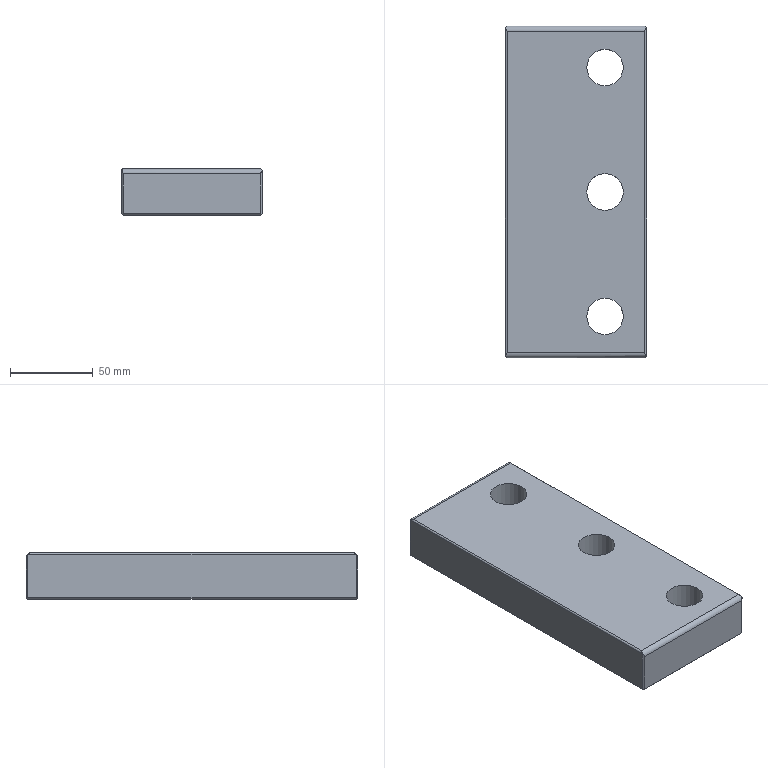Part | NX | features solid 2 | 1 solid | 21 faces | box 85 x 200 x 28 mm | volume 443266 mm3 | plane 15 | cylinder 6 | commonest cylinder face diameters 22 x3 6 x2 2 x1
STEP:
#1=CARTESIAN_POINT('',(590.,131.,-159.));
#2=VERTEX_POINT('',#1);
#3=CARTESIAN_POINT('',(590.,131.,-133.));
#4=VERTEX_POINT('',#3);
#5=CARTESIAN_POINT('',(590.,131.,-132.));
#6=DIRECTION('',(0.,0.,1.));
#7=VECTOR('',#6,1000.);
#8=LINE('',#5,#7);
#9=EDGE_CURVE('',#2,#4,#8,.T.);
#10=ORIENTED_EDGE('',*,*,#9,.T.);
#11=CARTESIAN_POINT('',(590.,329.,-133.));
#12=VERTEX_POINT('',#11);
#13=CARTESIAN_POINT('',(590.,350.,-133.));
#14=DIRECTION('',(0.,-1.,0.));
#15=VECTOR('',#14,1000.);
#16=LINE('',#13,#15);
#17=EDGE_CURVE('',#4,#12,#16,.F.);
#18=ORIENTED_EDGE('',*,*,#17,.T.);
#19=CARTESIAN_POINT('',(590.,329.,-159.));
#20=VERTEX_POINT('',#19);
#21=CARTESIAN_POINT('',(590.,329.,-132.));
#22=DIRECTION('',(0.,0.,-1.));
#23=VECTOR('',#22,1000.);
#24=LINE('',#21,#23);
#25=EDGE_CURVE('',#12,#20,#24,.T.);
#26=ORIENTED_EDGE('',*,*,#25,.T.);
#27=CARTESIAN_POINT('',(590.,350.,-159.));
#28=DIRECTION('',(0.,-1.,0.));
#29=VECTOR('',#28,1000.);
#30=LINE('',#27,#29);
#31=EDGE_CURVE('',#20,#2,#30,.T.);
#32=ORIENTED_EDGE('',*,*,#31,.T.);
#33=EDGE_LOOP('',(#10,#18,#26,#32));
#34=FACE_BOUND('',#33,.T.);
#35=CARTESIAN_POINT('',(590.,350.,-132.));
#36=DIRECTION('',(-1.,0.,0.));
#37=DIRECTION('',(0.,0.,1.));
#38=AXIS2_PLACEMENT_3D('',#35,#36,#37);
#39=PLANE('',#38);
#40=ADVANCED_FACE('',(#34),#39,.T.);
#41=CARTESIAN_POINT('',(639.,305.,-160.));
#42=VERTEX_POINT('',#41);
#43=CARTESIAN_POINT('',(650.,305.,-160.));
#44=DIRECTION('',(0.,0.,-1.));
#45=DIRECTION('',(-1.,0.,0.));
#46=AXIS2_PLACEMENT_3D('',#43,#44,#45);
#47=CIRCLE('',#46,11.);
#48=EDGE_CURVE('',#42,#42,#47,.T.);
#49=ORIENTED_EDGE('',*,*,#48,.F.);
#50=EDGE_LOOP('',(#49));
#51=FACE_BOUND('',#50,.T.);
#52=CARTESIAN_POINT('',(639.,230.,-160.));
#53=VERTEX_POINT('',#52);
#54=CARTESIAN_POINT('',(650.,230.,-160.));
#55=DIRECTION('',(0.,0.,-1.));
#56=DIRECTION('',(-1.,0.,0.));
#57=AXIS2_PLACEMENT_3D('',#54,#55,#56);
#58=CIRCLE('',#57,11.);
#59=EDGE_CURVE('',#53,#53,#58,.T.);
#60=ORIENTED_EDGE('',*,*,#59,.F.);
#61=EDGE_LOOP('',(#60));
#62=FACE_BOUND('',#61,.T.);
#63=CARTESIAN_POINT('',(639.,155.,-160.));
#64=VERTEX_POINT('',#63);
#65=CARTESIAN_POINT('',(650.,155.,-160.));
#66=DIRECTION('',(0.,0.,-1.));
#67=DIRECTION('',(-1.,0.,0.));
#68=AXIS2_PLACEMENT_3D('',#65,#66,#67);
#69=CIRCLE('',#68,11.);
#70=EDGE_CURVE('',#64,#64,#69,.T.);
#71=ORIENTED_EDGE('',*,*,#70,.F.);
#72=EDGE_LOOP('',(#71));
#73=FACE_BOUND('',#72,.T.);
#74=CARTESIAN_POINT('',(674.,329.,-160.));
#75=VERTEX_POINT('',#74);
#76=CARTESIAN_POINT('',(674.,131.,-160.));
#77=VERTEX_POINT('',#76);
#78=CARTESIAN_POINT('',(674.,350.,-160.));
#79=DIRECTION('',(0.,-1.,0.));
#80=VECTOR('',#79,1000.);
#81=LINE('',#78,#80);
#82=EDGE_CURVE('',#75,#77,#81,.T.);
#83=ORIENTED_EDGE('',*,*,#82,.T.);
#84=CARTESIAN_POINT('',(591.,131.,-160.));
#85=VERTEX_POINT('',#84);
#86=CARTESIAN_POINT('',(591.,131.,-160.));
#87=DIRECTION('',(-1.,0.,0.));
#88=VECTOR('',#87,1000.);
#89=LINE('',#86,#88);
#90=EDGE_CURVE('',#77,#85,#89,.T.);
#91=ORIENTED_EDGE('',*,*,#90,.T.);
#92=CARTESIAN_POINT('',(591.,329.,-160.));
#93=VERTEX_POINT('',#92);
#94=CARTESIAN_POINT('',(591.,350.,-160.));
#95=DIRECTION('',(0.,1.,0.));
#96=VECTOR('',#95,1000.);
#97=LINE('',#94,#96);
#98=EDGE_CURVE('',#85,#93,#97,.T.);
#99=ORIENTED_EDGE('',*,*,#98,.T.);
#100=CARTESIAN_POINT('',(590.,329.,-160.));
#101=DIRECTION('',(1.,0.,0.));
#102=VECTOR('',#101,1000.);
#103=LINE('',#100,#102);
#104=EDGE_CURVE('',#93,#75,#103,.T.);
#105=ORIENTED_EDGE('',*,*,#104,.T.);
#106=EDGE_LOOP('',(#83,#91,#99,#105));
#107=FACE_BOUND('',#106,.T.);
#108=CARTESIAN_POINT('',(590.,350.,-160.));
#109=DIRECTION('',(0.,0.,-1.));
#110=DIRECTION('',(-1.,0.,0.));
#111=AXIS2_PLACEMENT_3D('',#108,#109,#110);
#112=PLANE('',#111);
#113=ADVANCED_FACE('',(#51,#62,#73,#107),#112,.T.);
#114=CARTESIAN_POINT('',(675.,131.,-133.));
#115=VERTEX_POINT('',#114);
#116=CARTESIAN_POINT('',(675.,131.,-159.));
#117=VERTEX_POINT('',#116);
#118=CARTESIAN_POINT('',(675.,131.,-160.));
#119=DIRECTION('',(0.,0.,-1.));
#120=VECTOR('',#119,1000.);
#121=LINE('',#118,#120);
#122=EDGE_CURVE('',#115,#117,#121,.T.);
#123=ORIENTED_EDGE('',*,*,#122,.T.);
#124=CARTESIAN_POINT('',(675.,329.,-159.));
#125=VERTEX_POINT('',#124);
#126=CARTESIAN_POINT('',(675.,350.,-159.));
#127=DIRECTION('',(0.,1.,0.));
#128=VECTOR('',#127,1000.);
#129=LINE('',#126,#128);
#130=EDGE_CURVE('',#117,#125,#129,.T.);
#131=ORIENTED_EDGE('',*,*,#130,.T.);
#132=CARTESIAN_POINT('',(675.,329.,-133.));
#133=VERTEX_POINT('',#132);
#134=CARTESIAN_POINT('',(675.,329.,-160.));
#135=DIRECTION('',(0.,0.,1.));
#136=VECTOR('',#135,1000.);
#137=LINE('',#134,#136);
#138=EDGE_CURVE('',#125,#133,#137,.T.);
#139=ORIENTED_EDGE('',*,*,#138,.T.);
#140=CARTESIAN_POINT('',(675.,350.,-133.));
#141=DIRECTION('',(0.,-1.,0.));
#142=VECTOR('',#141,1000.);
#143=LINE('',#140,#142);
#144=EDGE_CURVE('',#133,#115,#143,.T.);
#145=ORIENTED_EDGE('',*,*,#144,.T.);
#146=EDGE_LOOP('',(#123,#131,#139,#145));
#147=FACE_BOUND('',#146,.T.);
#148=CARTESIAN_POINT('',(675.,350.,-160.));
#149=DIRECTION('',(1.,0.,0.));
#150=DIRECTION('',(0.,0.,-1.));
#151=AXIS2_PLACEMENT_3D('',#148,#149,#150);
#152=PLANE('',#151);
#153=ADVANCED_FACE('',(#147),#152,.T.);
#154=CARTESIAN_POINT('',(639.,305.,-132.));
#155=VERTEX_POINT('',#154);
#156=CARTESIAN_POINT('',(650.,305.,-132.));
#157=DIRECTION('',(0.,0.,-1.));
#158=DIRECTION('',(-1.,0.,0.));
#159=AXIS2_PLACEMENT_3D('',#156,#157,#158);
#160=CIRCLE('',#159,11.);
#161=EDGE_CURVE('',#155,#155,#160,.T.);
#162=ORIENTED_EDGE('',*,*,#161,.T.);
#163=EDGE_LOOP('',(#162));
#164=FACE_BOUND('',#163,.T.);
#165=CARTESIAN_POINT('',(639.,230.,-132.));
#166=VERTEX_POINT('',#165);
#167=CARTESIAN_POINT('',(650.,230.,-132.));
#168=DIRECTION('',(0.,0.,-1.));
#169=DIRECTION('',(-1.,0.,0.));
#170=AXIS2_PLACEMENT_3D('',#167,#168,#169);
#171=CIRCLE('',#170,11.);
#172=EDGE_CURVE('',#166,#166,#171,.T.);
#173=ORIENTED_EDGE('',*,*,#172,.T.);
#174=EDGE_LOOP('',(#173));
#175=FACE_BOUND('',#174,.T.);
#176=CARTESIAN_POINT('',(639.,155.,-132.));
#177=VERTEX_POINT('',#176);
#178=CARTESIAN_POINT('',(650.,155.,-132.));
#179=DIRECTION('',(0.,0.,-1.));
#180=DIRECTION('',(-1.,0.,0.));
#181=AXIS2_PLACEMENT_3D('',#178,#179,#180);
#182=CIRCLE('',#181,11.);
#183=EDGE_CURVE('',#177,#177,#182,.T.);
#184=ORIENTED_EDGE('',*,*,#183,.T.);
#185=EDGE_LOOP('',(#184));
#186=FACE_BOUND('',#185,.T.);
#187=CARTESIAN_POINT('',(674.,133.,-132.));
#188=VERTEX_POINT('',#187);
#189=CARTESIAN_POINT('',(674.,327.,-132.));
#190=VERTEX_POINT('',#189);
#191=CARTESIAN_POINT('',(674.,350.,-132.));
#192=DIRECTION('',(0.,1.,0.));
#193=VECTOR('',#192,1000.);
#194=LINE('',#191,#193);
#195=EDGE_CURVE('',#188,#190,#194,.T.);
#196=ORIENTED_EDGE('',*,*,#195,.T.);
#197=CARTESIAN_POINT('',(591.,327.,-132.));
#198=VERTEX_POINT('',#197);
#199=CARTESIAN_POINT('',(675.,327.,-132.));
#200=DIRECTION('',(-1.,0.,0.));
#201=VECTOR('',#200,1000.);
#202=LINE('',#199,#201);
#203=EDGE_CURVE('',#190,#198,#202,.T.);
#204=ORIENTED_EDGE('',*,*,#203,.T.);
#205=CARTESIAN_POINT('',(591.,133.,-132.));
#206=VERTEX_POINT('',#205);
#207=CARTESIAN_POINT('',(591.,350.,-132.));
#208=DIRECTION('',(0.,-1.,0.));
#209=VECTOR('',#208,1000.);
#210=LINE('',#207,#209);
#211=EDGE_CURVE('',#198,#206,#210,.T.);
#212=ORIENTED_EDGE('',*,*,#211,.T.);
#213=CARTESIAN_POINT('',(674.,133.,-132.));
#214=DIRECTION('',(-1.,0.,0.));
#215=VECTOR('',#214,1000.);
#216=LINE('',#213,#215);
#217=EDGE_CURVE('',#206,#188,#216,.F.);
#218=ORIENTED_EDGE('',*,*,#217,.T.);
#219=EDGE_LOOP('',(#196,#204,#212,#218));
#220=FACE_BOUND('',#219,.T.);
#221=CARTESIAN_POINT('',(675.,350.,-132.));
#222=DIRECTION('',(0.,0.,1.));
#223=DIRECTION('',(1.,0.,0.));
#224=AXIS2_PLACEMENT_3D('',#221,#222,#223);
#225=PLANE('',#224);
#226=ADVANCED_FACE('',(#164,#175,#186,#220),#225,.T.);
#227=CARTESIAN_POINT('',(674.,330.,-135.));
#228=VERTEX_POINT('',#227);
#229=CARTESIAN_POINT('',(674.,330.,-159.));
#230=VERTEX_POINT('',#229);
#231=CARTESIAN_POINT('',(674.,330.,-132.));
#232=DIRECTION('',(0.,0.,-1.));
#233=VECTOR('',#232,1000.);
#234=LINE('',#231,#233);
#235=EDGE_CURVE('',#228,#230,#234,.T.);
#236=ORIENTED_EDGE('',*,*,#235,.T.);
#237=CARTESIAN_POINT('',(591.,330.,-159.));
#238=VERTEX_POINT('',#237);
#239=CARTESIAN_POINT('',(590.,330.,-159.));
#240=DIRECTION('',(-1.,0.,0.));
#241=VECTOR('',#240,1000.);
#242=LINE('',#239,#241);
#243=EDGE_CURVE('',#230,#238,#242,.T.);
#244=ORIENTED_EDGE('',*,*,#243,.T.);
#245=CARTESIAN_POINT('',(591.,330.,-135.));
#246=VERTEX_POINT('',#245);
#247=CARTESIAN_POINT('',(591.,330.,-132.));
#248=DIRECTION('',(0.,0.,1.));
#249=VECTOR('',#248,1000.);
#250=LINE('',#247,#249);
#251=EDGE_CURVE('',#238,#246,#250,.T.);
#252=ORIENTED_EDGE('',*,*,#251,.T.);
#253=CARTESIAN_POINT('',(590.,330.,-135.));
#254=DIRECTION('',(-1.,0.,0.));
#255=VECTOR('',#254,1000.);
#256=LINE('',#253,#255);
#257=EDGE_CURVE('',#246,#228,#256,.F.);
#258=ORIENTED_EDGE('',*,*,#257,.T.);
#259=EDGE_LOOP('',(#236,#244,#252,#258));
#260=FACE_BOUND('',#259,.T.);
#261=CARTESIAN_POINT('',(590.,330.,-132.));
#262=DIRECTION('',(0.,1.,0.));
#263=DIRECTION('',(0.,0.,-1.));
#264=AXIS2_PLACEMENT_3D('',#261,#262,#263);
#265=PLANE('',#264);
#266=ADVANCED_FACE('',(#260),#265,.T.);
#267=CARTESIAN_POINT('',(591.,130.,-135.));
#268=VERTEX_POINT('',#267);
#269=CARTESIAN_POINT('',(591.,130.,-159.));
#270=VERTEX_POINT('',#269);
#271=CARTESIAN_POINT('',(591.,130.,-160.));
#272=DIRECTION('',(0.,0.,-1.));
#273=VECTOR('',#272,1000.);
#274=LINE('',#271,#273);
#275=EDGE_CURVE('',#268,#270,#274,.T.);
#276=ORIENTED_EDGE('',*,*,#275,.T.);
#277=CARTESIAN_POINT('',(674.,130.,-159.));
#278=VERTEX_POINT('',#277);
#279=CARTESIAN_POINT('',(674.,130.,-159.));
#280=DIRECTION('',(1.,0.,0.));
#281=VECTOR('',#280,1000.);
#282=LINE('',#279,#281);
#283=EDGE_CURVE('',#270,#278,#282,.T.);
#284=ORIENTED_EDGE('',*,*,#283,.T.);
#285=CARTESIAN_POINT('',(674.,130.,-135.));
#286=VERTEX_POINT('',#285);
#287=CARTESIAN_POINT('',(674.,130.,-132.));
#288=DIRECTION('',(0.,0.,1.));
#289=VECTOR('',#288,1000.);
#290=LINE('',#287,#289);
#291=EDGE_CURVE('',#278,#286,#290,.T.);
#292=ORIENTED_EDGE('',*,*,#291,.T.);
#293=CARTESIAN_POINT('',(591.,130.,-135.));
#294=DIRECTION('',(-1.,0.,0.));
#295=VECTOR('',#294,1000.);
#296=LINE('',#293,#295);
#297=EDGE_CURVE('',#286,#268,#296,.T.);
#298=ORIENTED_EDGE('',*,*,#297,.T.);
#299=EDGE_LOOP('',(#276,#284,#292,#298));
#300=FACE_BOUND('',#299,.T.);
#301=CARTESIAN_POINT('',(590.,130.,-132.));
#302=DIRECTION('',(0.,1.,0.));
#303=DIRECTION('',(0.,0.,-1.));
#304=AXIS2_PLACEMENT_3D('',#301,#302,#303);
#305=PLANE('',#304);
#306=ADVANCED_FACE('',(#300),#305,.F.);
#307=ORIENTED_EDGE('',*,*,#70,.T.);
#308=EDGE_LOOP('',(#307));
#309=FACE_BOUND('',#308,.T.);
#310=ORIENTED_EDGE('',*,*,#183,.F.);
#311=EDGE_LOOP('',(#310));
#312=FACE_BOUND('',#311,.T.);
#313=CARTESIAN_POINT('',(650.,155.,-132.));
#314=DIRECTION('',(0.,0.,-1.));
#315=DIRECTION('',(-1.,0.,0.));
#316=AXIS2_PLACEMENT_3D('',#313,#314,#315);
#317=CYLINDRICAL_SURFACE('',#316,11.);
#318=ADVANCED_FACE('',(#309,#312),#317,.F.);
#319=ORIENTED_EDGE('',*,*,#251,.F.);
#320=CARTESIAN_POINT('',(590.5,329.5,-159.5));
#321=VERTEX_POINT('',#320);
#322=CARTESIAN_POINT('',(599.333,338.333,-150.667));
#323=DIRECTION('',(-0.5774,-0.5774,-0.5774));
#324=VECTOR('',#323,1000.);
#325=LINE('',#322,#324);
#326=EDGE_CURVE('',#238,#321,#325,.T.);
#327=ORIENTED_EDGE('',*,*,#326,.T.);
#328=CARTESIAN_POINT('',(581.,320.,-150.));
#329=DIRECTION('',(-0.5774,-0.5774,0.5774));
#330=VECTOR('',#329,1000.);
#331=LINE('',#328,#330);
#332=EDGE_CURVE('',#321,#20,#331,.T.);
#333=ORIENTED_EDGE('',*,*,#332,.T.);
#334=ORIENTED_EDGE('',*,*,#25,.F.);
#335=CARTESIAN_POINT('',(590.023,329.023,-132.785));
#336=VERTEX_POINT('',#335);
#337=CARTESIAN_POINT('',(591.,330.,-133.));
#338=DIRECTION('',(0.7071,-0.7071,0.));
#339=DIRECTION('',(-0.7071,-0.7071,0.));
#340=AXIS2_PLACEMENT_3D('',#337,#338,#339);
#341=ELLIPSE('',#340,1.414,1.);
#342=EDGE_CURVE('',#12,#336,#341,.F.);
#343=ORIENTED_EDGE('',*,*,#342,.T.);
#344=CARTESIAN_POINT('',(588.,327.,-135.));
#345=DIRECTION('',(0.7071,-0.7071,0.));
#346=DIRECTION('',(-0.7071,-0.7071,0.));
#347=AXIS2_PLACEMENT_3D('',#344,#345,#346);
#348=ELLIPSE('',#347,4.243,3.);
#349=EDGE_CURVE('',#336,#246,#348,.F.);
#350=ORIENTED_EDGE('',*,*,#349,.T.);
#351=EDGE_LOOP('',(#319,#327,#333,#334,#343,#350));
#352=FACE_BOUND('',#351,.T.);
#353=CARTESIAN_POINT('',(590.,329.,-132.));
#354=DIRECTION('',(0.7071,-0.7071,0.));
#355=DIRECTION('',(0.7071,0.7071,0.));
#356=AXIS2_PLACEMENT_3D('',#353,#354,#355);
#357=PLANE('',#356);
#358=ADVANCED_FACE('',(#352),#357,.F.);
#359=CARTESIAN_POINT('',(674.5,329.5,-159.5));
#360=VERTEX_POINT('',#359);
#361=CARTESIAN_POINT('',(674.667,329.333,-159.333));
#362=DIRECTION('',(-0.5774,0.5774,-0.5774));
#363=VECTOR('',#362,1000.);
#364=LINE('',#361,#363);
#365=EDGE_CURVE('',#125,#360,#364,.T.);
#366=ORIENTED_EDGE('',*,*,#365,.T.);
#367=CARTESIAN_POINT('',(675.,329.,-160.));
#368=DIRECTION('',(-0.5774,0.5774,0.5774));
#369=VECTOR('',#368,1000.);
#370=LINE('',#367,#369);
#371=EDGE_CURVE('',#360,#230,#370,.T.);
#372=ORIENTED_EDGE('',*,*,#371,.T.);
#373=ORIENTED_EDGE('',*,*,#235,.F.);
#374=CARTESIAN_POINT('',(674.879,329.121,-132.879));
#375=VERTEX_POINT('',#374);
#376=CARTESIAN_POINT('',(677.,327.,-135.));
#377=DIRECTION('',(-0.7071,-0.7071,0.));
#378=DIRECTION('',(-0.7071,0.7071,0.));
#379=AXIS2_PLACEMENT_3D('',#376,#377,#378);
#380=ELLIPSE('',#379,4.243,3.);
#381=EDGE_CURVE('',#228,#375,#380,.F.);
#382=ORIENTED_EDGE('',*,*,#381,.T.);
#383=CARTESIAN_POINT('',(684.,320.,-142.));
#384=DIRECTION('',(0.5774,-0.5774,-0.5774));
#385=VECTOR('',#384,1000.);
#386=LINE('',#383,#385);
#387=EDGE_CURVE('',#375,#133,#386,.T.);
#388=ORIENTED_EDGE('',*,*,#387,.T.);
#389=ORIENTED_EDGE('',*,*,#138,.F.);
#390=EDGE_LOOP('',(#366,#372,#373,#382,#388,#389));
#391=FACE_BOUND('',#390,.T.);
#392=CARTESIAN_POINT('',(675.,329.,-160.));
#393=DIRECTION('',(-0.7071,-0.7071,0.));
#394=DIRECTION('',(0.7071,-0.7071,0.));
#395=AXIS2_PLACEMENT_3D('',#392,#393,#394);
#396=PLANE('',#395);
#397=ADVANCED_FACE('',(#391),#396,.F.);
#398=CARTESIAN_POINT('',(590.023,130.977,-132.785));
#399=VERTEX_POINT('',#398);
#400=CARTESIAN_POINT('',(588.,133.,-135.));
#401=DIRECTION('',(-0.7071,-0.7071,0.));
#402=DIRECTION('',(0.7071,-0.7071,0.));
#403=AXIS2_PLACEMENT_3D('',#400,#401,#402);
#404=ELLIPSE('',#403,4.243,3.);
#405=EDGE_CURVE('',#268,#399,#404,.T.);
#406=ORIENTED_EDGE('',*,*,#405,.T.);
#407=CARTESIAN_POINT('',(591.,130.,-133.));
#408=DIRECTION('',(-0.7071,-0.7071,0.));
#409=DIRECTION('',(0.7071,-0.7071,0.));
#410=AXIS2_PLACEMENT_3D('',#407,#408,#409);
#411=ELLIPSE('',#410,1.414,1.);
#412=EDGE_CURVE('',#399,#4,#411,.T.);
#413=ORIENTED_EDGE('',*,*,#412,.T.);
#414=ORIENTED_EDGE('',*,*,#9,.F.);
#415=CARTESIAN_POINT('',(590.5,130.5,-159.5));
#416=VERTEX_POINT('',#415);
#417=CARTESIAN_POINT('',(581.667,139.333,-150.667));
#418=DIRECTION('',(-0.5774,0.5774,0.5774));
#419=VECTOR('',#418,1000.);
#420=LINE('',#417,#419);
#421=EDGE_CURVE('',#2,#416,#420,.F.);
#422=ORIENTED_EDGE('',*,*,#421,.T.);
#423=CARTESIAN_POINT('',(600.,121.,-150.));
#424=DIRECTION('',(0.5774,-0.5774,0.5774));
#425=VECTOR('',#424,1000.);
#426=LINE('',#423,#425);
#427=EDGE_CURVE('',#416,#270,#426,.T.);
#428=ORIENTED_EDGE('',*,*,#427,.T.);
#429=ORIENTED_EDGE('',*,*,#275,.F.);
#430=EDGE_LOOP('',(#406,#413,#414,#422,#428,#429));
#431=FACE_BOUND('',#430,.T.);
#432=CARTESIAN_POINT('',(591.,130.,-132.));
#433=DIRECTION('',(-0.7071,-0.7071,0.));
#434=DIRECTION('',(0.7071,-0.7071,0.));
#435=AXIS2_PLACEMENT_3D('',#432,#433,#434);
#436=PLANE('',#435);
#437=ADVANCED_FACE('',(#431),#436,.T.);
#438=ORIENTED_EDGE('',*,*,#291,.F.);
#439=CARTESIAN_POINT('',(674.5,130.5,-159.5));
#440=VERTEX_POINT('',#439);
#441=CARTESIAN_POINT('',(665.,121.,-150.));
#442=DIRECTION('',(0.5774,0.5774,-0.5774));
#443=VECTOR('',#442,1000.);
#444=LINE('',#441,#443);
#445=EDGE_CURVE('',#278,#440,#444,.T.);
#446=ORIENTED_EDGE('',*,*,#445,.T.);
#447=CARTESIAN_POINT('',(683.333,139.333,-150.667));
#448=DIRECTION('',(-0.5774,-0.5774,-0.5774));
#449=VECTOR('',#448,1000.);
#450=LINE('',#447,#449);
#451=EDGE_CURVE('',#440,#117,#450,.F.);
#452=ORIENTED_EDGE('',*,*,#451,.T.);
#453=ORIENTED_EDGE('',*,*,#122,.F.);
#454=CARTESIAN_POINT('',(674.879,130.879,-132.879));
#455=VERTEX_POINT('',#454);
#456=CARTESIAN_POINT('',(674.,130.,-132.));
#457=DIRECTION('',(0.5774,0.5774,-0.5774));
#458=VECTOR('',#457,1000.);
#459=LINE('',#456,#458);
#460=EDGE_CURVE('',#115,#455,#459,.F.);
#461=ORIENTED_EDGE('',*,*,#460,.T.);
#462=CARTESIAN_POINT('',(677.,133.,-135.));
#463=DIRECTION('',(0.7071,-0.7071,0.));
#464=DIRECTION('',(0.7071,0.7071,0.));
#465=AXIS2_PLACEMENT_3D('',#462,#463,#464);
#466=ELLIPSE('',#465,4.243,3.);
#467=EDGE_CURVE('',#455,#286,#466,.T.);
#468=ORIENTED_EDGE('',*,*,#467,.T.);
#469=EDGE_LOOP('',(#438,#446,#452,#453,#461,#468));
#470=FACE_BOUND('',#469,.T.);
#471=CARTESIAN_POINT('',(674.,130.,-132.));
#472=DIRECTION('',(0.7071,-0.7071,0.));
#473=DIRECTION('',(0.7071,0.7071,0.));
#474=AXIS2_PLACEMENT_3D('',#471,#472,#473);
#475=PLANE('',#474);
#476=ADVANCED_FACE('',(#470),#475,.T.);
#477=ORIENTED_EDGE('',*,*,#98,.F.);
#478=CARTESIAN_POINT('',(656.667,196.667,-225.667));
#479=DIRECTION('',(0.5774,0.5774,-0.5774));
#480=VECTOR('',#479,1000.);
#481=LINE('',#478,#480);
#482=EDGE_CURVE('',#85,#416,#481,.F.);
#483=ORIENTED_EDGE('',*,*,#482,.T.);
#484=ORIENTED_EDGE('',*,*,#421,.F.);
#485=ORIENTED_EDGE('',*,*,#31,.F.);
#486=ORIENTED_EDGE('',*,*,#332,.F.);
#487=CARTESIAN_POINT('',(590.,330.,-159.));
#488=DIRECTION('',(0.5774,-0.5774,-0.5774));
#489=VECTOR('',#488,1000.);
#490=LINE('',#487,#489);
#491=EDGE_CURVE('',#321,#93,#490,.T.);
#492=ORIENTED_EDGE('',*,*,#491,.T.);
#493=EDGE_LOOP('',(#477,#483,#484,#485,#486,#492));
#494=FACE_BOUND('',#493,.T.);
#495=CARTESIAN_POINT('',(590.,350.,-159.));
#496=DIRECTION('',(0.7071,0.,0.7071));
#497=DIRECTION('',(0.7071,0.,-0.7071));
#498=AXIS2_PLACEMENT_3D('',#495,#496,#497);
#499=PLANE('',#498);
#500=ADVANCED_FACE('',(#494),#499,.F.);
#501=ORIENTED_EDGE('',*,*,#451,.F.);
#502=CARTESIAN_POINT('',(607.667,197.333,-226.333));
#503=DIRECTION('',(0.5774,-0.5774,0.5774));
#504=VECTOR('',#503,1000.);
#505=LINE('',#502,#504);
#506=EDGE_CURVE('',#440,#77,#505,.F.);
#507=ORIENTED_EDGE('',*,*,#506,.T.);
#508=ORIENTED_EDGE('',*,*,#82,.F.);
#509=CARTESIAN_POINT('',(674.333,329.333,-159.667));
#510=DIRECTION('',(0.5774,0.5774,0.5774));
#511=VECTOR('',#510,1000.);
#512=LINE('',#509,#511);
#513=EDGE_CURVE('',#75,#360,#512,.T.);
#514=ORIENTED_EDGE('',*,*,#513,.T.);
#515=ORIENTED_EDGE('',*,*,#365,.F.);
#516=ORIENTED_EDGE('',*,*,#130,.F.);
#517=EDGE_LOOP('',(#501,#507,#508,#514,#515,#516));
#518=FACE_BOUND('',#517,.T.);
#519=CARTESIAN_POINT('',(674.,350.,-160.));
#520=DIRECTION('',(-0.7071,0.,0.7071));
#521=DIRECTION('',(0.7071,0.,0.7071));
#522=AXIS2_PLACEMENT_3D('',#519,#520,#521);
#523=PLANE('',#522);
#524=ADVANCED_FACE('',(#518),#523,.F.);
#525=ORIENTED_EDGE('',*,*,#387,.F.);
#526=CARTESIAN_POINT('',(677.,327.,-135.));
#527=DIRECTION('',(-0.7071,0.,-0.7071));
#528=DIRECTION('',(-0.7071,0.,0.7071));
#529=AXIS2_PLACEMENT_3D('',#526,#527,#528);
#530=ELLIPSE('',#529,4.243,3.);
#531=EDGE_CURVE('',#375,#190,#530,.F.);
#532=ORIENTED_EDGE('',*,*,#531,.T.);
#533=ORIENTED_EDGE('',*,*,#195,.F.);
#534=CARTESIAN_POINT('',(677.,133.,-135.));
#535=DIRECTION('',(-0.7071,0.,-0.7071));
#536=DIRECTION('',(0.7071,0.,-0.7071));
#537=AXIS2_PLACEMENT_3D('',#534,#535,#536);
#538=ELLIPSE('',#537,4.243,3.);
#539=EDGE_CURVE('',#188,#455,#538,.F.);
#540=ORIENTED_EDGE('',*,*,#539,.T.);
#541=ORIENTED_EDGE('',*,*,#460,.F.);
#542=ORIENTED_EDGE('',*,*,#144,.F.);
#543=EDGE_LOOP('',(#525,#532,#533,#540,#541,#542));
#544=FACE_BOUND('',#543,.T.);
#545=CARTESIAN_POINT('',(675.,350.,-133.));
#546=DIRECTION('',(-0.7071,0.,-0.7071));
#547=DIRECTION('',(-0.7071,0.,0.7071));
#548=AXIS2_PLACEMENT_3D('',#545,#546,#547);
#549=PLANE('',#548);
#550=ADVANCED_FACE('',(#544),#549,.F.);
#551=ORIENTED_EDGE('',*,*,#211,.F.);
#552=CARTESIAN_POINT('',(590.023,329.023,-132.785));
#553=CARTESIAN_POINT('',(590.144,328.423,-132.236));
#554=CARTESIAN_POINT('',(590.595,327.702,-132.));
#555=CARTESIAN_POINT('',(591.,327.,-132.));
#556=B_SPLINE_CURVE_WITH_KNOTS('',3,(#552,#553,#554,#555),.UNSPECIFIED.,.F.,.F.,(4,4),(0.,0.002432),.UNSPECIFIED.);
#557=EDGE_CURVE('',#198,#336,#556,.F.);
#558=ORIENTED_EDGE('',*,*,#557,.T.);
#559=ORIENTED_EDGE('',*,*,#342,.F.);
#560=ORIENTED_EDGE('',*,*,#17,.F.);
#561=ORIENTED_EDGE('',*,*,#412,.F.);
#562=CARTESIAN_POINT('',(590.023,130.977,-132.785));
#563=CARTESIAN_POINT('',(590.144,131.577,-132.236));
#564=CARTESIAN_POINT('',(590.595,132.298,-132.));
#565=CARTESIAN_POINT('',(591.,133.,-132.));
#566=B_SPLINE_CURVE_WITH_KNOTS('',3,(#562,#563,#564,#565),.UNSPECIFIED.,.F.,.F.,(4,4),(0.,0.002432),.UNSPECIFIED.);
#567=EDGE_CURVE('',#399,#206,#566,.T.);
#568=ORIENTED_EDGE('',*,*,#567,.T.);
#569=EDGE_LOOP('',(#551,#558,#559,#560,#561,#568));
#570=FACE_BOUND('',#569,.T.);
#571=CARTESIAN_POINT('',(591.,350.,-133.));
#572=DIRECTION('',(0.,-1.,0.));
#573=DIRECTION('',(0.,0.,1.));
#574=AXIS2_PLACEMENT_3D('',#571,#572,#573);
#575=CYLINDRICAL_SURFACE('',#574,1.);
#576=ADVANCED_FACE('',(#570),#575,.T.);
#577=ORIENTED_EDGE('',*,*,#59,.T.);
#578=EDGE_LOOP('',(#577));
#579=FACE_BOUND('',#578,.T.);
#580=ORIENTED_EDGE('',*,*,#172,.F.);
#581=EDGE_LOOP('',(#580));
#582=FACE_BOUND('',#581,.T.);
#583=CARTESIAN_POINT('',(650.,230.,-132.));
#584=DIRECTION('',(0.,0.,-1.));
#585=DIRECTION('',(-1.,0.,0.));
#586=AXIS2_PLACEMENT_3D('',#583,#584,#585);
#587=CYLINDRICAL_SURFACE('',#586,11.);
#588=ADVANCED_FACE('',(#579,#582),#587,.F.);
#589=ORIENTED_EDGE('',*,*,#48,.T.);
#590=EDGE_LOOP('',(#589));
#591=FACE_BOUND('',#590,.T.);
#592=ORIENTED_EDGE('',*,*,#161,.F.);
#593=EDGE_LOOP('',(#592));
#594=FACE_BOUND('',#593,.T.);
#595=CARTESIAN_POINT('',(650.,305.,-132.));
#596=DIRECTION('',(0.,0.,-1.));
#597=DIRECTION('',(-1.,0.,0.));
#598=AXIS2_PLACEMENT_3D('',#595,#596,#597);
#599=CYLINDRICAL_SURFACE('',#598,11.);
#600=ADVANCED_FACE('',(#591,#594),#599,.F.);
#601=ORIENTED_EDGE('',*,*,#381,.F.);
#602=ORIENTED_EDGE('',*,*,#257,.F.);
#603=ORIENTED_EDGE('',*,*,#349,.F.);
#604=ORIENTED_EDGE('',*,*,#557,.F.);
#605=ORIENTED_EDGE('',*,*,#203,.F.);
#606=ORIENTED_EDGE('',*,*,#531,.F.);
#607=EDGE_LOOP('',(#601,#602,#603,#604,#605,#606));
#608=FACE_BOUND('',#607,.T.);
#609=CARTESIAN_POINT('',(675.,327.,-135.));
#610=DIRECTION('',(-1.,0.,0.));
#611=DIRECTION('',(0.,0.,1.));
#612=AXIS2_PLACEMENT_3D('',#609,#610,#611);
#613=CYLINDRICAL_SURFACE('',#612,3.);
#614=ADVANCED_FACE('',(#608),#613,.T.);
#615=ORIENTED_EDGE('',*,*,#567,.F.);
#616=ORIENTED_EDGE('',*,*,#405,.F.);
#617=ORIENTED_EDGE('',*,*,#297,.F.);
#618=ORIENTED_EDGE('',*,*,#467,.F.);
#619=ORIENTED_EDGE('',*,*,#539,.F.);
#620=ORIENTED_EDGE('',*,*,#217,.F.);
#621=EDGE_LOOP('',(#615,#616,#617,#618,#619,#620));
#622=FACE_BOUND('',#621,.T.);
#623=CARTESIAN_POINT('',(590.,133.,-135.));
#624=DIRECTION('',(1.,0.,0.));
#625=DIRECTION('',(0.,0.,-1.));
#626=AXIS2_PLACEMENT_3D('',#623,#624,#625);
#627=CYLINDRICAL_SURFACE('',#626,3.);
#628=ADVANCED_FACE('',(#622),#627,.T.);
#629=ORIENTED_EDGE('',*,*,#482,.F.);
#630=ORIENTED_EDGE('',*,*,#90,.F.);
#631=ORIENTED_EDGE('',*,*,#506,.F.);
#632=ORIENTED_EDGE('',*,*,#445,.F.);
#633=ORIENTED_EDGE('',*,*,#283,.F.);
#634=ORIENTED_EDGE('',*,*,#427,.F.);
#635=EDGE_LOOP('',(#629,#630,#631,#632,#633,#634));
#636=FACE_BOUND('',#635,.T.);
#637=CARTESIAN_POINT('',(590.,130.,-159.));
#638=DIRECTION('',(0.,-0.7071,-0.7071));
#639=DIRECTION('',(0.,-0.7071,0.7071));
#640=AXIS2_PLACEMENT_3D('',#637,#638,#639);
#641=PLANE('',#640);
#642=ADVANCED_FACE('',(#636),#641,.T.);
#643=ORIENTED_EDGE('',*,*,#326,.F.);
#644=ORIENTED_EDGE('',*,*,#243,.F.);
#645=ORIENTED_EDGE('',*,*,#371,.F.);
#646=ORIENTED_EDGE('',*,*,#513,.F.);
#647=ORIENTED_EDGE('',*,*,#104,.F.);
#648=ORIENTED_EDGE('',*,*,#491,.F.);
#649=EDGE_LOOP('',(#643,#644,#645,#646,#647,#648));
#650=FACE_BOUND('',#649,.T.);
#651=CARTESIAN_POINT('',(590.,329.,-160.));
#652=DIRECTION('',(0.,-0.7071,0.7071));
#653=DIRECTION('',(0.,0.7071,0.7071));
#654=AXIS2_PLACEMENT_3D('',#651,#652,#653);
#655=PLANE('',#654);
#656=ADVANCED_FACE('',(#650),#655,.F.);
#657=CLOSED_SHELL('',(#40,#113,#153,#226,#266,#306,#318,#358,#397,#437,#476,#500,#524,#550,#576,#588,#600,#614,#628,#642,#656));
#658=MANIFOLD_SOLID_BREP('',#657);
#659=(LENGTH_UNIT()NAMED_UNIT(*)SI_UNIT(.MILLI.,.METRE.));
#660=UNCERTAINTY_MEASURE_WITH_UNIT(LENGTH_MEASURE(0.0508),#659,'','');
#661=(NAMED_UNIT(*)PLANE_ANGLE_UNIT()SI_UNIT($,.RADIAN.));
#662=(NAMED_UNIT(*)SI_UNIT($,.STERADIAN.)SOLID_ANGLE_UNIT());
#663=(GEOMETRIC_REPRESENTATION_CONTEXT(3)GLOBAL_UNCERTAINTY_ASSIGNED_CONTEXT((#660))GLOBAL_UNIT_ASSIGNED_CONTEXT((#659,#661,#662))REPRESENTATION_CONTEXT('',''));
#664=ADVANCED_BREP_SHAPE_REPRESENTATION('',(#658),#663);